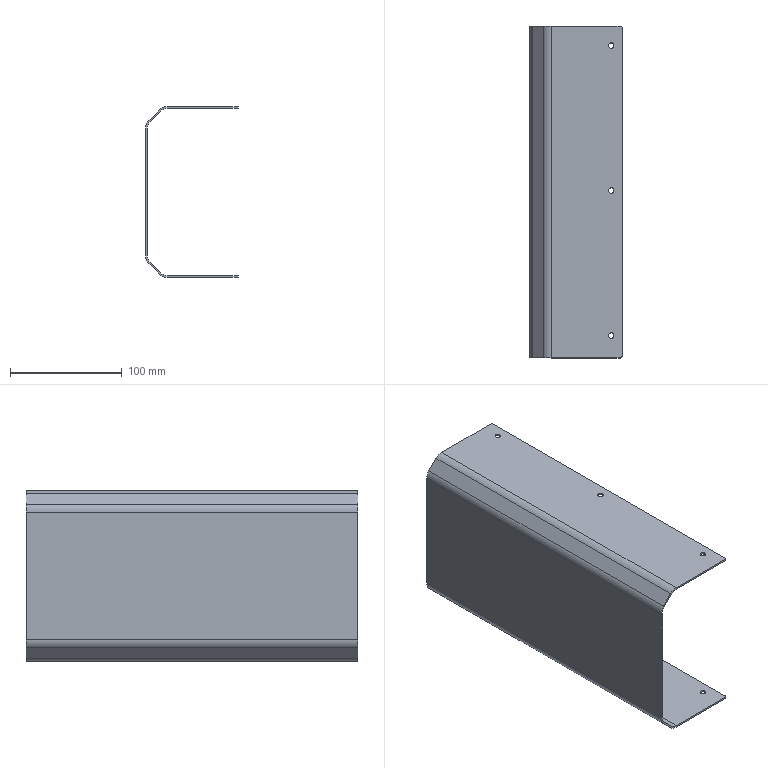Part | SolidWorks | features ICE 3, Fillet 2, Shell 2, Chamfer 1, Extrusion 1, HoleWzd 1 | 1 solid | 38 faces | box 83 x 297.5 x 153 mm | volume 132510 mm3 | cylinder 24 | plane 14 | commonest cylinder face diameters 5 x12 4 x4 17 x4 20 x4
STEP:
#1=CARTESIAN_POINT('',(29.,-17.5,75.));
#2=VERTEX_POINT('',#1);
#3=CARTESIAN_POINT('',(34.,-17.5,75.));
#4=VERTEX_POINT('',#3);
#5=CARTESIAN_POINT('',(31.5,-17.5,75.));
#6=DIRECTION('',(0.,0.,1.));
#7=DIRECTION('',(1.,0.,0.));
#8=AXIS2_PLACEMENT_3D('',#5,#6,#7);
#9=CIRCLE('',#8,2.5);
#10=EDGE_CURVE('',#2,#4,#9,.T.);
#11=ORIENTED_EDGE('',*,*,#10,.F.);
#12=CARTESIAN_POINT('',(29.,-17.5,76.5));
#13=VERTEX_POINT('',#12);
#14=CARTESIAN_POINT('',(29.,-17.5,76.5));
#15=DIRECTION('',(0.,0.,1.));
#16=VECTOR('',#15,1000.);
#17=LINE('',#14,#16);
#18=EDGE_CURVE('',#2,#13,#17,.T.);
#19=ORIENTED_EDGE('',*,*,#18,.T.);
#20=CARTESIAN_POINT('',(34.,-17.5,76.5));
#21=VERTEX_POINT('',#20);
#22=CARTESIAN_POINT('',(31.5,-17.5,76.5));
#23=DIRECTION('',(0.,0.,1.));
#24=DIRECTION('',(1.,0.,0.));
#25=AXIS2_PLACEMENT_3D('',#22,#23,#24);
#26=CIRCLE('',#25,2.5);
#27=EDGE_CURVE('',#13,#21,#26,.T.);
#28=ORIENTED_EDGE('',*,*,#27,.T.);
#29=CARTESIAN_POINT('',(34.,-17.5,76.5));
#30=DIRECTION('',(0.,0.,1.));
#31=VECTOR('',#30,1000.);
#32=LINE('',#29,#31);
#33=EDGE_CURVE('',#4,#21,#32,.T.);
#34=ORIENTED_EDGE('',*,*,#33,.F.);
#35=EDGE_LOOP('',(#11,#19,#28,#34));
#36=FACE_OUTER_BOUND('',#35,.T.);
#37=CARTESIAN_POINT('',(31.5,-17.5,76.5));
#38=DIRECTION('',(0.,0.,1.));
#39=DIRECTION('',(1.,0.,0.));
#40=AXIS2_PLACEMENT_3D('',#37,#38,#39);
#41=CYLINDRICAL_SURFACE('',#40,2.5);
#42=ADVANCED_FACE('',(#36),#41,.F.);
#43=CARTESIAN_POINT('',(29.,-17.5,-76.5));
#44=VERTEX_POINT('',#43);
#45=CARTESIAN_POINT('',(34.,-17.5,-76.5));
#46=VERTEX_POINT('',#45);
#47=CARTESIAN_POINT('',(31.5,-17.5,-76.5));
#48=DIRECTION('',(0.,0.,1.));
#49=DIRECTION('',(1.,0.,0.));
#50=AXIS2_PLACEMENT_3D('',#47,#48,#49);
#51=CIRCLE('',#50,2.5);
#52=EDGE_CURVE('',#44,#46,#51,.T.);
#53=ORIENTED_EDGE('',*,*,#52,.F.);
#54=CARTESIAN_POINT('',(29.,-17.5,-75.));
#55=VERTEX_POINT('',#54);
#56=CARTESIAN_POINT('',(29.,-17.5,76.5));
#57=DIRECTION('',(0.,0.,1.));
#58=VECTOR('',#57,1000.);
#59=LINE('',#56,#58);
#60=EDGE_CURVE('',#44,#55,#59,.T.);
#61=ORIENTED_EDGE('',*,*,#60,.T.);
#62=CARTESIAN_POINT('',(34.,-17.5,-75.));
#63=VERTEX_POINT('',#62);
#64=CARTESIAN_POINT('',(31.5,-17.5,-75.));
#65=DIRECTION('',(0.,0.,-1.));
#66=DIRECTION('',(-1.,0.,0.));
#67=AXIS2_PLACEMENT_3D('',#64,#65,#66);
#68=CIRCLE('',#67,2.5);
#69=EDGE_CURVE('',#63,#55,#68,.T.);
#70=ORIENTED_EDGE('',*,*,#69,.F.);
#71=CARTESIAN_POINT('',(34.,-17.5,76.5));
#72=DIRECTION('',(0.,0.,1.));
#73=VECTOR('',#72,1000.);
#74=LINE('',#71,#73);
#75=EDGE_CURVE('',#46,#63,#74,.T.);
#76=ORIENTED_EDGE('',*,*,#75,.F.);
#77=EDGE_LOOP('',(#53,#61,#70,#76));
#78=FACE_OUTER_BOUND('',#77,.T.);
#79=CARTESIAN_POINT('',(31.5,-17.5,76.5));
#80=DIRECTION('',(0.,0.,1.));
#81=DIRECTION('',(1.,0.,0.));
#82=AXIS2_PLACEMENT_3D('',#79,#80,#81);
#83=CYLINDRICAL_SURFACE('',#82,2.5);
#84=ADVANCED_FACE('',(#78),#83,.F.);
#85=CARTESIAN_POINT('',(29.,-147.5,75.));
#86=VERTEX_POINT('',#85);
#87=CARTESIAN_POINT('',(34.,-147.5,75.));
#88=VERTEX_POINT('',#87);
#89=CARTESIAN_POINT('',(31.5,-147.5,75.));
#90=DIRECTION('',(0.,0.,1.));
#91=DIRECTION('',(1.,0.,0.));
#92=AXIS2_PLACEMENT_3D('',#89,#90,#91);
#93=CIRCLE('',#92,2.5);
#94=EDGE_CURVE('',#86,#88,#93,.T.);
#95=ORIENTED_EDGE('',*,*,#94,.F.);
#96=CARTESIAN_POINT('',(29.,-147.5,76.5));
#97=VERTEX_POINT('',#96);
#98=CARTESIAN_POINT('',(29.,-147.5,76.5));
#99=DIRECTION('',(0.,0.,1.));
#100=VECTOR('',#99,1000.);
#101=LINE('',#98,#100);
#102=EDGE_CURVE('',#86,#97,#101,.T.);
#103=ORIENTED_EDGE('',*,*,#102,.T.);
#104=CARTESIAN_POINT('',(34.,-147.5,76.5));
#105=VERTEX_POINT('',#104);
#106=CARTESIAN_POINT('',(31.5,-147.5,76.5));
#107=DIRECTION('',(0.,0.,1.));
#108=DIRECTION('',(1.,0.,0.));
#109=AXIS2_PLACEMENT_3D('',#106,#107,#108);
#110=CIRCLE('',#109,2.5);
#111=EDGE_CURVE('',#97,#105,#110,.T.);
#112=ORIENTED_EDGE('',*,*,#111,.T.);
#113=CARTESIAN_POINT('',(34.,-147.5,76.5));
#114=DIRECTION('',(0.,0.,1.));
#115=VECTOR('',#114,1000.);
#116=LINE('',#113,#115);
#117=EDGE_CURVE('',#88,#105,#116,.T.);
#118=ORIENTED_EDGE('',*,*,#117,.F.);
#119=EDGE_LOOP('',(#95,#103,#112,#118));
#120=FACE_OUTER_BOUND('',#119,.T.);
#121=CARTESIAN_POINT('',(31.5,-147.5,76.5));
#122=DIRECTION('',(0.,0.,1.));
#123=DIRECTION('',(1.,0.,0.));
#124=AXIS2_PLACEMENT_3D('',#121,#122,#123);
#125=CYLINDRICAL_SURFACE('',#124,2.5);
#126=ADVANCED_FACE('',(#120),#125,.F.);
#127=CARTESIAN_POINT('',(29.,-147.5,-76.5));
#128=VERTEX_POINT('',#127);
#129=CARTESIAN_POINT('',(34.,-147.5,-76.5));
#130=VERTEX_POINT('',#129);
#131=CARTESIAN_POINT('',(31.5,-147.5,-76.5));
#132=DIRECTION('',(0.,0.,1.));
#133=DIRECTION('',(1.,0.,0.));
#134=AXIS2_PLACEMENT_3D('',#131,#132,#133);
#135=CIRCLE('',#134,2.5);
#136=EDGE_CURVE('',#128,#130,#135,.T.);
#137=ORIENTED_EDGE('',*,*,#136,.F.);
#138=CARTESIAN_POINT('',(29.,-147.5,-75.));
#139=VERTEX_POINT('',#138);
#140=CARTESIAN_POINT('',(29.,-147.5,76.5));
#141=DIRECTION('',(0.,0.,1.));
#142=VECTOR('',#141,1000.);
#143=LINE('',#140,#142);
#144=EDGE_CURVE('',#128,#139,#143,.T.);
#145=ORIENTED_EDGE('',*,*,#144,.T.);
#146=CARTESIAN_POINT('',(34.,-147.5,-75.));
#147=VERTEX_POINT('',#146);
#148=CARTESIAN_POINT('',(31.5,-147.5,-75.));
#149=DIRECTION('',(0.,0.,-1.));
#150=DIRECTION('',(-1.,0.,0.));
#151=AXIS2_PLACEMENT_3D('',#148,#149,#150);
#152=CIRCLE('',#151,2.5);
#153=EDGE_CURVE('',#147,#139,#152,.T.);
#154=ORIENTED_EDGE('',*,*,#153,.F.);
#155=CARTESIAN_POINT('',(34.,-147.5,76.5));
#156=DIRECTION('',(0.,0.,1.));
#157=VECTOR('',#156,1000.);
#158=LINE('',#155,#157);
#159=EDGE_CURVE('',#130,#147,#158,.T.);
#160=ORIENTED_EDGE('',*,*,#159,.F.);
#161=EDGE_LOOP('',(#137,#145,#154,#160));
#162=FACE_OUTER_BOUND('',#161,.T.);
#163=CARTESIAN_POINT('',(31.5,-147.5,76.5));
#164=DIRECTION('',(0.,0.,1.));
#165=DIRECTION('',(1.,0.,0.));
#166=AXIS2_PLACEMENT_3D('',#163,#164,#165);
#167=CYLINDRICAL_SURFACE('',#166,2.5);
#168=ADVANCED_FACE('',(#162),#167,.F.);
#169=CARTESIAN_POINT('',(29.,-277.5,75.));
#170=VERTEX_POINT('',#169);
#171=CARTESIAN_POINT('',(34.,-277.5,75.));
#172=VERTEX_POINT('',#171);
#173=CARTESIAN_POINT('',(31.5,-277.5,75.));
#174=DIRECTION('',(0.,0.,1.));
#175=DIRECTION('',(1.,0.,0.));
#176=AXIS2_PLACEMENT_3D('',#173,#174,#175);
#177=CIRCLE('',#176,2.5);
#178=EDGE_CURVE('',#170,#172,#177,.T.);
#179=ORIENTED_EDGE('',*,*,#178,.F.);
#180=CARTESIAN_POINT('',(29.,-277.5,76.5));
#181=VERTEX_POINT('',#180);
#182=CARTESIAN_POINT('',(29.,-277.5,76.5));
#183=DIRECTION('',(0.,0.,1.));
#184=VECTOR('',#183,1000.);
#185=LINE('',#182,#184);
#186=EDGE_CURVE('',#170,#181,#185,.T.);
#187=ORIENTED_EDGE('',*,*,#186,.T.);
#188=CARTESIAN_POINT('',(34.,-277.5,76.5));
#189=VERTEX_POINT('',#188);
#190=CARTESIAN_POINT('',(31.5,-277.5,76.5));
#191=DIRECTION('',(0.,0.,1.));
#192=DIRECTION('',(1.,0.,0.));
#193=AXIS2_PLACEMENT_3D('',#190,#191,#192);
#194=CIRCLE('',#193,2.5);
#195=EDGE_CURVE('',#181,#189,#194,.T.);
#196=ORIENTED_EDGE('',*,*,#195,.T.);
#197=CARTESIAN_POINT('',(34.,-277.5,76.5));
#198=DIRECTION('',(0.,0.,1.));
#199=VECTOR('',#198,1000.);
#200=LINE('',#197,#199);
#201=EDGE_CURVE('',#172,#189,#200,.T.);
#202=ORIENTED_EDGE('',*,*,#201,.F.);
#203=EDGE_LOOP('',(#179,#187,#196,#202));
#204=FACE_OUTER_BOUND('',#203,.T.);
#205=CARTESIAN_POINT('',(31.5,-277.5,76.5));
#206=DIRECTION('',(0.,0.,1.));
#207=DIRECTION('',(1.,0.,0.));
#208=AXIS2_PLACEMENT_3D('',#205,#206,#207);
#209=CYLINDRICAL_SURFACE('',#208,2.5);
#210=ADVANCED_FACE('',(#204),#209,.F.);
#211=CARTESIAN_POINT('',(29.,-277.5,-76.5));
#212=VERTEX_POINT('',#211);
#213=CARTESIAN_POINT('',(34.,-277.5,-76.5));
#214=VERTEX_POINT('',#213);
#215=CARTESIAN_POINT('',(31.5,-277.5,-76.5));
#216=DIRECTION('',(0.,0.,1.));
#217=DIRECTION('',(1.,0.,0.));
#218=AXIS2_PLACEMENT_3D('',#215,#216,#217);
#219=CIRCLE('',#218,2.5);
#220=EDGE_CURVE('',#212,#214,#219,.T.);
#221=ORIENTED_EDGE('',*,*,#220,.F.);
#222=CARTESIAN_POINT('',(29.,-277.5,-75.));
#223=VERTEX_POINT('',#222);
#224=CARTESIAN_POINT('',(29.,-277.5,76.5));
#225=DIRECTION('',(0.,0.,1.));
#226=VECTOR('',#225,1000.);
#227=LINE('',#224,#226);
#228=EDGE_CURVE('',#212,#223,#227,.T.);
#229=ORIENTED_EDGE('',*,*,#228,.T.);
#230=CARTESIAN_POINT('',(34.,-277.5,-75.));
#231=VERTEX_POINT('',#230);
#232=CARTESIAN_POINT('',(31.5,-277.5,-75.));
#233=DIRECTION('',(0.,0.,-1.));
#234=DIRECTION('',(-1.,0.,0.));
#235=AXIS2_PLACEMENT_3D('',#232,#233,#234);
#236=CIRCLE('',#235,2.5);
#237=EDGE_CURVE('',#231,#223,#236,.T.);
#238=ORIENTED_EDGE('',*,*,#237,.F.);
#239=CARTESIAN_POINT('',(34.,-277.5,76.5));
#240=DIRECTION('',(0.,0.,1.));
#241=VECTOR('',#240,1000.);
#242=LINE('',#239,#241);
#243=EDGE_CURVE('',#214,#231,#242,.T.);
#244=ORIENTED_EDGE('',*,*,#243,.F.);
#245=EDGE_LOOP('',(#221,#229,#238,#244));
#246=FACE_OUTER_BOUND('',#245,.T.);
#247=CARTESIAN_POINT('',(31.5,-277.5,76.5));
#248=DIRECTION('',(0.,0.,1.));
#249=DIRECTION('',(1.,0.,0.));
#250=AXIS2_PLACEMENT_3D('',#247,#248,#249);
#251=CYLINDRICAL_SURFACE('',#250,2.5);
#252=ADVANCED_FACE('',(#246),#251,.F.);
#253=CARTESIAN_POINT('',(41.5,-295.5,76.5));
#254=VERTEX_POINT('',#253);
#255=CARTESIAN_POINT('',(41.5,-2.,76.5));
#256=VERTEX_POINT('',#255);
#257=CARTESIAN_POINT('',(41.5,-297.5,76.5));
#258=DIRECTION('',(0.,1.,0.));
#259=VECTOR('',#258,1000.);
#260=LINE('',#257,#259);
#261=EDGE_CURVE('',#254,#256,#260,.T.);
#262=ORIENTED_EDGE('',*,*,#261,.F.);
#263=CARTESIAN_POINT('',(41.5,-295.5,75.));
#264=VERTEX_POINT('',#263);
#265=CARTESIAN_POINT('',(41.5,-295.5,75.));
#266=DIRECTION('',(0.,0.,-1.));
#267=VECTOR('',#266,1000.);
#268=LINE('',#265,#267);
#269=EDGE_CURVE('',#254,#264,#268,.T.);
#270=ORIENTED_EDGE('',*,*,#269,.T.);
#271=CARTESIAN_POINT('',(41.5,-2.,75.));
#272=VERTEX_POINT('',#271);
#273=CARTESIAN_POINT('',(41.5,-297.5,75.));
#274=DIRECTION('',(0.,1.,0.));
#275=VECTOR('',#274,1000.);
#276=LINE('',#273,#275);
#277=EDGE_CURVE('',#264,#272,#276,.T.);
#278=ORIENTED_EDGE('',*,*,#277,.T.);
#279=CARTESIAN_POINT('',(41.5,-2.,-76.5));
#280=DIRECTION('',(0.,0.,1.));
#281=VECTOR('',#280,1000.);
#282=LINE('',#279,#281);
#283=EDGE_CURVE('',#272,#256,#282,.T.);
#284=ORIENTED_EDGE('',*,*,#283,.T.);
#285=EDGE_LOOP('',(#262,#270,#278,#284));
#286=FACE_OUTER_BOUND('',#285,.T.);
#287=CARTESIAN_POINT('',(41.5,-297.5,-76.5));
#288=DIRECTION('',(1.,0.,0.));
#289=DIRECTION('',(0.,0.,-1.));
#290=AXIS2_PLACEMENT_3D('',#287,#288,#289);
#291=PLANE('',#290);
#292=ADVANCED_FACE('',(#286),#291,.T.);
#293=CARTESIAN_POINT('',(41.5,-295.5,-75.));
#294=VERTEX_POINT('',#293);
#295=CARTESIAN_POINT('',(41.5,-2.,-75.));
#296=VERTEX_POINT('',#295);
#297=CARTESIAN_POINT('',(41.5,-297.5,-75.));
#298=DIRECTION('',(0.,1.,0.));
#299=VECTOR('',#298,1000.);
#300=LINE('',#297,#299);
#301=EDGE_CURVE('',#294,#296,#300,.T.);
#302=ORIENTED_EDGE('',*,*,#301,.F.);
#303=CARTESIAN_POINT('',(41.5,-295.5,-76.5));
#304=VERTEX_POINT('',#303);
#305=CARTESIAN_POINT('',(41.5,-295.5,-76.5));
#306=DIRECTION('',(0.,0.,-1.));
#307=VECTOR('',#306,1000.);
#308=LINE('',#305,#307);
#309=EDGE_CURVE('',#294,#304,#308,.T.);
#310=ORIENTED_EDGE('',*,*,#309,.T.);
#311=CARTESIAN_POINT('',(41.5,-2.,-76.5));
#312=VERTEX_POINT('',#311);
#313=CARTESIAN_POINT('',(41.5,-297.5,-76.5));
#314=DIRECTION('',(0.,1.,0.));
#315=VECTOR('',#314,1000.);
#316=LINE('',#313,#315);
#317=EDGE_CURVE('',#304,#312,#316,.T.);
#318=ORIENTED_EDGE('',*,*,#317,.T.);
#319=CARTESIAN_POINT('',(41.5,-2.,-76.5));
#320=DIRECTION('',(0.,0.,1.));
#321=VECTOR('',#320,1000.);
#322=LINE('',#319,#321);
#323=EDGE_CURVE('',#312,#296,#322,.T.);
#324=ORIENTED_EDGE('',*,*,#323,.T.);
#325=EDGE_LOOP('',(#302,#310,#318,#324));
#326=FACE_OUTER_BOUND('',#325,.T.);
#327=CARTESIAN_POINT('',(41.5,-297.5,-76.5));
#328=DIRECTION('',(1.,0.,0.));
#329=DIRECTION('',(0.,0.,-1.));
#330=AXIS2_PLACEMENT_3D('',#327,#328,#329);
#331=PLANE('',#330);
#332=ADVANCED_FACE('',(#326),#331,.T.);
#333=CARTESIAN_POINT('',(31.5,-17.5,76.5));
#334=DIRECTION('',(0.,0.,1.));
#335=DIRECTION('',(1.,0.,0.));
#336=AXIS2_PLACEMENT_3D('',#333,#334,#335);
#337=CIRCLE('',#336,2.5);
#338=EDGE_CURVE('',#21,#13,#337,.T.);
#339=ORIENTED_EDGE('',*,*,#338,.F.);
#340=ORIENTED_EDGE('',*,*,#27,.F.);
#341=EDGE_LOOP('',(#339,#340));
#342=FACE_BOUND('',#341,.T.);
#343=CARTESIAN_POINT('',(31.5,-147.5,76.5));
#344=DIRECTION('',(0.,0.,1.));
#345=DIRECTION('',(1.,0.,0.));
#346=AXIS2_PLACEMENT_3D('',#343,#344,#345);
#347=CIRCLE('',#346,2.5);
#348=EDGE_CURVE('',#105,#97,#347,.T.);
#349=ORIENTED_EDGE('',*,*,#348,.F.);
#350=ORIENTED_EDGE('',*,*,#111,.F.);
#351=EDGE_LOOP('',(#349,#350));
#352=FACE_BOUND('',#351,.T.);
#353=CARTESIAN_POINT('',(31.5,-277.5,76.5));
#354=DIRECTION('',(0.,0.,1.));
#355=DIRECTION('',(1.,0.,0.));
#356=AXIS2_PLACEMENT_3D('',#353,#354,#355);
#357=CIRCLE('',#356,2.5);
#358=EDGE_CURVE('',#189,#181,#357,.T.);
#359=ORIENTED_EDGE('',*,*,#358,.F.);
#360=ORIENTED_EDGE('',*,*,#195,.F.);
#361=EDGE_LOOP('',(#359,#360));
#362=FACE_BOUND('',#361,.T.);
#363=CARTESIAN_POINT('',(-22.358,-297.5,76.5));
#364=VERTEX_POINT('',#363);
#365=CARTESIAN_POINT('',(39.5,-297.5,76.5));
#366=VERTEX_POINT('',#365);
#367=CARTESIAN_POINT('',(-41.5,-297.5,76.5));
#368=DIRECTION('',(1.,0.,0.));
#369=VECTOR('',#368,1000.);
#370=LINE('',#367,#369);
#371=EDGE_CURVE('',#364,#366,#370,.T.);
#372=ORIENTED_EDGE('',*,*,#371,.T.);
#373=CARTESIAN_POINT('',(39.5,-295.5,76.5));
#374=DIRECTION('',(0.,0.,1.));
#375=DIRECTION('',(1.,0.,0.));
#376=AXIS2_PLACEMENT_3D('',#373,#374,#375);
#377=CIRCLE('',#376,2.);
#378=EDGE_CURVE('',#366,#254,#377,.T.);
#379=ORIENTED_EDGE('',*,*,#378,.T.);
#380=ORIENTED_EDGE('',*,*,#261,.T.);
#381=CARTESIAN_POINT('',(39.5,0.,76.5));
#382=VERTEX_POINT('',#381);
#383=CARTESIAN_POINT('',(39.5,-2.,76.5));
#384=DIRECTION('',(0.,0.,1.));
#385=DIRECTION('',(1.,0.,0.));
#386=AXIS2_PLACEMENT_3D('',#383,#384,#385);
#387=CIRCLE('',#386,2.);
#388=EDGE_CURVE('',#256,#382,#387,.T.);
#389=ORIENTED_EDGE('',*,*,#388,.T.);
#390=CARTESIAN_POINT('',(-22.358,0.,76.5));
#391=VERTEX_POINT('',#390);
#392=CARTESIAN_POINT('',(-41.5,0.,76.5));
#393=DIRECTION('',(1.,0.,0.));
#394=VECTOR('',#393,1000.);
#395=LINE('',#392,#394);
#396=EDGE_CURVE('',#391,#382,#395,.T.);
#397=ORIENTED_EDGE('',*,*,#396,.F.);
#398=CARTESIAN_POINT('',(-22.358,-297.5,76.5));
#399=DIRECTION('',(0.,-1.,0.));
#400=VECTOR('',#399,1000.);
#401=LINE('',#398,#400);
#402=EDGE_CURVE('',#391,#364,#401,.T.);
#403=ORIENTED_EDGE('',*,*,#402,.T.);
#404=EDGE_LOOP('',(#372,#379,#380,#389,#397,#403));
#405=FACE_OUTER_BOUND('',#404,.T.);
#406=CARTESIAN_POINT('',(-41.5,-297.5,76.5));
#407=DIRECTION('',(0.,0.,1.));
#408=DIRECTION('',(1.,0.,0.));
#409=AXIS2_PLACEMENT_3D('',#406,#407,#408);
#410=PLANE('',#409);
#411=ADVANCED_FACE('',(#342,#352,#362,#405),#410,.T.);
#412=CARTESIAN_POINT('',(-41.5,0.,-57.358));
#413=VERTEX_POINT('',#412);
#414=CARTESIAN_POINT('',(-41.5,0.,57.358));
#415=VERTEX_POINT('',#414);
#416=CARTESIAN_POINT('',(-41.5,0.,-76.5));
#417=DIRECTION('',(0.,0.,1.));
#418=VECTOR('',#417,1000.);
#419=LINE('',#416,#418);
#420=EDGE_CURVE('',#413,#415,#419,.T.);
#421=ORIENTED_EDGE('',*,*,#420,.F.);
#422=CARTESIAN_POINT('',(-41.5,-297.5,-57.358));
#423=VERTEX_POINT('',#422);
#424=CARTESIAN_POINT('',(-41.5,-297.5,-57.358));
#425=DIRECTION('',(0.,-1.,0.));
#426=VECTOR('',#425,1000.);
#427=LINE('',#424,#426);
#428=EDGE_CURVE('',#413,#423,#427,.T.);
#429=ORIENTED_EDGE('',*,*,#428,.T.);
#430=CARTESIAN_POINT('',(-41.5,-297.5,57.358));
#431=VERTEX_POINT('',#430);
#432=CARTESIAN_POINT('',(-41.5,-297.5,-76.5));
#433=DIRECTION('',(0.,0.,1.));
#434=VECTOR('',#433,1000.);
#435=LINE('',#432,#434);
#436=EDGE_CURVE('',#423,#431,#435,.T.);
#437=ORIENTED_EDGE('',*,*,#436,.T.);
#438=CARTESIAN_POINT('',(-41.5,-297.5,57.358));
#439=DIRECTION('',(0.,1.,0.));
#440=VECTOR('',#439,1000.);
#441=LINE('',#438,#440);
#442=EDGE_CURVE('',#431,#415,#441,.T.);
#443=ORIENTED_EDGE('',*,*,#442,.T.);
#444=EDGE_LOOP('',(#421,#429,#437,#443));
#445=FACE_OUTER_BOUND('',#444,.T.);
#446=CARTESIAN_POINT('',(-41.5,-297.5,-76.5));
#447=DIRECTION('',(-1.,0.,0.));
#448=DIRECTION('',(0.,0.,1.));
#449=AXIS2_PLACEMENT_3D('',#446,#447,#448);
#450=PLANE('',#449);
#451=ADVANCED_FACE('',(#445),#450,.T.);
#452=CARTESIAN_POINT('',(31.5,-17.5,-76.5));
#453=DIRECTION('',(0.,0.,1.));
#454=DIRECTION('',(1.,0.,0.));
#455=AXIS2_PLACEMENT_3D('',#452,#453,#454);
#456=CIRCLE('',#455,2.5);
#457=EDGE_CURVE('',#46,#44,#456,.T.);
#458=ORIENTED_EDGE('',*,*,#457,.T.);
#459=ORIENTED_EDGE('',*,*,#52,.T.);
#460=EDGE_LOOP('',(#458,#459));
#461=FACE_BOUND('',#460,.T.);
#462=CARTESIAN_POINT('',(31.5,-147.5,-76.5));
#463=DIRECTION('',(0.,0.,1.));
#464=DIRECTION('',(1.,0.,0.));
#465=AXIS2_PLACEMENT_3D('',#462,#463,#464);
#466=CIRCLE('',#465,2.5);
#467=EDGE_CURVE('',#130,#128,#466,.T.);
#468=ORIENTED_EDGE('',*,*,#467,.T.);
#469=ORIENTED_EDGE('',*,*,#136,.T.);
#470=EDGE_LOOP('',(#468,#469));
#471=FACE_BOUND('',#470,.T.);
#472=CARTESIAN_POINT('',(31.5,-277.5,-76.5));
#473=DIRECTION('',(0.,0.,1.));
#474=DIRECTION('',(1.,0.,0.));
#475=AXIS2_PLACEMENT_3D('',#472,#473,#474);
#476=CIRCLE('',#475,2.5);
#477=EDGE_CURVE('',#214,#212,#476,.T.);
#478=ORIENTED_EDGE('',*,*,#477,.T.);
#479=ORIENTED_EDGE('',*,*,#220,.T.);
#480=EDGE_LOOP('',(#478,#479));
#481=FACE_BOUND('',#480,.T.);
#482=ORIENTED_EDGE('',*,*,#317,.F.);
#483=CARTESIAN_POINT('',(39.5,-297.5,-76.5));
#484=VERTEX_POINT('',#483);
#485=CARTESIAN_POINT('',(39.5,-295.5,-76.5));
#486=DIRECTION('',(0.,0.,-1.));
#487=DIRECTION('',(-1.,0.,0.));
#488=AXIS2_PLACEMENT_3D('',#485,#486,#487);
#489=CIRCLE('',#488,2.);
#490=EDGE_CURVE('',#304,#484,#489,.T.);
#491=ORIENTED_EDGE('',*,*,#490,.T.);
#492=CARTESIAN_POINT('',(-22.358,-297.5,-76.5));
#493=VERTEX_POINT('',#492);
#494=CARTESIAN_POINT('',(-41.5,-297.5,-76.5));
#495=DIRECTION('',(-1.,0.,0.));
#496=VECTOR('',#495,1000.);
#497=LINE('',#494,#496);
#498=EDGE_CURVE('',#484,#493,#497,.T.);
#499=ORIENTED_EDGE('',*,*,#498,.T.);
#500=CARTESIAN_POINT('',(-22.358,0.,-76.5));
#501=VERTEX_POINT('',#500);
#502=CARTESIAN_POINT('',(-22.358,-297.5,-76.5));
#503=DIRECTION('',(0.,1.,0.));
#504=VECTOR('',#503,1000.);
#505=LINE('',#502,#504);
#506=EDGE_CURVE('',#493,#501,#505,.T.);
#507=ORIENTED_EDGE('',*,*,#506,.T.);
#508=CARTESIAN_POINT('',(39.5,0.,-76.5));
#509=VERTEX_POINT('',#508);
#510=CARTESIAN_POINT('',(-41.5,0.,-76.5));
#511=DIRECTION('',(-1.,0.,0.));
#512=VECTOR('',#511,1000.);
#513=LINE('',#510,#512);
#514=EDGE_CURVE('',#509,#501,#513,.T.);
#515=ORIENTED_EDGE('',*,*,#514,.F.);
#516=CARTESIAN_POINT('',(39.5,-2.,-76.5));
#517=DIRECTION('',(0.,0.,-1.));
#518=DIRECTION('',(-1.,0.,0.));
#519=AXIS2_PLACEMENT_3D('',#516,#517,#518);
#520=CIRCLE('',#519,2.);
#521=EDGE_CURVE('',#509,#312,#520,.T.);
#522=ORIENTED_EDGE('',*,*,#521,.T.);
#523=EDGE_LOOP('',(#482,#491,#499,#507,#515,#522));
#524=FACE_OUTER_BOUND('',#523,.T.);
#525=CARTESIAN_POINT('',(-41.5,-297.5,-76.5));
#526=DIRECTION('',(0.,0.,-1.));
#527=DIRECTION('',(-1.,0.,0.));
#528=AXIS2_PLACEMENT_3D('',#525,#526,#527);
#529=PLANE('',#528);
#530=ADVANCED_FACE('',(#461,#471,#481,#524),#529,.T.);
#531=ORIENTED_EDGE('',*,*,#498,.F.);
#532=CARTESIAN_POINT('',(39.5,-297.5,-75.));
#533=VERTEX_POINT('',#532);
#534=CARTESIAN_POINT('',(39.5,-297.5,-75.));
#535=DIRECTION('',(0.,0.,1.));
#536=VECTOR('',#535,1000.);
#537=LINE('',#534,#536);
#538=EDGE_CURVE('',#484,#533,#537,.T.);
#539=ORIENTED_EDGE('',*,*,#538,.T.);
#540=CARTESIAN_POINT('',(-22.358,-297.5,-75.));
#541=VERTEX_POINT('',#540);
#542=CARTESIAN_POINT('',(0.,-297.5,-75.));
#543=DIRECTION('',(-1.,0.,0.));
#544=VECTOR('',#543,1000.);
#545=LINE('',#542,#544);
#546=EDGE_CURVE('',#533,#541,#545,.T.);
#547=ORIENTED_EDGE('',*,*,#546,.T.);
#548=CARTESIAN_POINT('',(-28.368,-297.5,-72.51));
#549=VERTEX_POINT('',#548);
#550=CARTESIAN_POINT('',(-22.358,-297.5,-66.5));
#551=DIRECTION('',(0.,-1.,0.));
#552=DIRECTION('',(0.,0.,1.));
#553=AXIS2_PLACEMENT_3D('',#550,#551,#552);
#554=CIRCLE('',#553,8.5);
#555=EDGE_CURVE('',#549,#541,#554,.T.);
#556=ORIENTED_EDGE('',*,*,#555,.F.);
#557=CARTESIAN_POINT('',(-37.51,-297.5,-63.368));
#558=VERTEX_POINT('',#557);
#559=CARTESIAN_POINT('',(-25.439,-297.5,-75.439));
#560=DIRECTION('',(0.7071,0.,-0.7071));
#561=VECTOR('',#560,1000.);
#562=LINE('',#559,#561);
#563=EDGE_CURVE('',#558,#549,#562,.T.);
#564=ORIENTED_EDGE('',*,*,#563,.F.);
#565=CARTESIAN_POINT('',(-40.,-297.5,-57.358));
#566=VERTEX_POINT('',#565);
#567=CARTESIAN_POINT('',(-31.5,-297.5,-57.358));
#568=DIRECTION('',(0.,-1.,0.));
#569=DIRECTION('',(0.,0.,1.));
#570=AXIS2_PLACEMENT_3D('',#567,#568,#569);
#571=CIRCLE('',#570,8.5);
#572=EDGE_CURVE('',#566,#558,#571,.T.);
#573=ORIENTED_EDGE('',*,*,#572,.F.);
#574=CARTESIAN_POINT('',(-40.,-297.5,57.358));
#575=VERTEX_POINT('',#574);
#576=CARTESIAN_POINT('',(-40.,-297.5,0.));
#577=DIRECTION('',(0.,0.,1.));
#578=VECTOR('',#577,1000.);
#579=LINE('',#576,#578);
#580=EDGE_CURVE('',#566,#575,#579,.T.);
#581=ORIENTED_EDGE('',*,*,#580,.T.);
#582=CARTESIAN_POINT('',(-37.51,-297.5,63.368));
#583=VERTEX_POINT('',#582);
#584=CARTESIAN_POINT('',(-31.5,-297.5,57.358));
#585=DIRECTION('',(0.,-1.,0.));
#586=DIRECTION('',(0.,0.,1.));
#587=AXIS2_PLACEMENT_3D('',#584,#585,#586);
#588=CIRCLE('',#587,8.5);
#589=EDGE_CURVE('',#583,#575,#588,.T.);
#590=ORIENTED_EDGE('',*,*,#589,.F.);
#591=CARTESIAN_POINT('',(-28.368,-297.5,72.51));
#592=VERTEX_POINT('',#591);
#593=CARTESIAN_POINT('',(-40.439,-297.5,60.439));
#594=DIRECTION('',(-0.7071,0.,-0.7071));
#595=VECTOR('',#594,1000.);
#596=LINE('',#593,#595);
#597=EDGE_CURVE('',#592,#583,#596,.T.);
#598=ORIENTED_EDGE('',*,*,#597,.F.);
#599=CARTESIAN_POINT('',(-22.358,-297.5,75.));
#600=VERTEX_POINT('',#599);
#601=CARTESIAN_POINT('',(-22.358,-297.5,66.5));
#602=DIRECTION('',(0.,-1.,0.));
#603=DIRECTION('',(0.,0.,1.));
#604=AXIS2_PLACEMENT_3D('',#601,#602,#603);
#605=CIRCLE('',#604,8.5);
#606=EDGE_CURVE('',#600,#592,#605,.T.);
#607=ORIENTED_EDGE('',*,*,#606,.F.);
#608=CARTESIAN_POINT('',(39.5,-297.5,75.));
#609=VERTEX_POINT('',#608);
#610=CARTESIAN_POINT('',(0.,-297.5,75.));
#611=DIRECTION('',(1.,0.,0.));
#612=VECTOR('',#611,1000.);
#613=LINE('',#610,#612);
#614=EDGE_CURVE('',#600,#609,#613,.T.);
#615=ORIENTED_EDGE('',*,*,#614,.T.);
#616=CARTESIAN_POINT('',(39.5,-297.5,76.5));
#617=DIRECTION('',(0.,0.,1.));
#618=VECTOR('',#617,1000.);
#619=LINE('',#616,#618);
#620=EDGE_CURVE('',#609,#366,#619,.T.);
#621=ORIENTED_EDGE('',*,*,#620,.T.);
#622=ORIENTED_EDGE('',*,*,#371,.F.);
#623=CARTESIAN_POINT('',(-29.429,-297.5,73.571));
#624=VERTEX_POINT('',#623);
#625=CARTESIAN_POINT('',(-22.358,-297.5,66.5));
#626=DIRECTION('',(0.,-1.,0.));
#627=DIRECTION('',(0.,0.,1.));
#628=AXIS2_PLACEMENT_3D('',#625,#626,#627);
#629=CIRCLE('',#628,10.);
#630=EDGE_CURVE('',#364,#624,#629,.T.);
#631=ORIENTED_EDGE('',*,*,#630,.T.);
#632=CARTESIAN_POINT('',(-38.571,-297.5,64.429));
#633=VERTEX_POINT('',#632);
#634=CARTESIAN_POINT('',(-41.5,-297.5,61.5));
#635=DIRECTION('',(-0.7071,0.,-0.7071));
#636=VECTOR('',#635,1000.);
#637=LINE('',#634,#636);
#638=EDGE_CURVE('',#624,#633,#637,.T.);
#639=ORIENTED_EDGE('',*,*,#638,.T.);
#640=CARTESIAN_POINT('',(-31.5,-297.5,57.358));
#641=DIRECTION('',(0.,-1.,0.));
#642=DIRECTION('',(0.,0.,1.));
#643=AXIS2_PLACEMENT_3D('',#640,#641,#642);
#644=CIRCLE('',#643,10.);
#645=EDGE_CURVE('',#633,#431,#644,.T.);
#646=ORIENTED_EDGE('',*,*,#645,.T.);
#647=ORIENTED_EDGE('',*,*,#436,.F.);
#648=CARTESIAN_POINT('',(-38.571,-297.5,-64.429));
#649=VERTEX_POINT('',#648);
#650=CARTESIAN_POINT('',(-31.5,-297.5,-57.358));
#651=DIRECTION('',(0.,-1.,0.));
#652=DIRECTION('',(0.,0.,1.));
#653=AXIS2_PLACEMENT_3D('',#650,#651,#652);
#654=CIRCLE('',#653,10.);
#655=EDGE_CURVE('',#423,#649,#654,.T.);
#656=ORIENTED_EDGE('',*,*,#655,.T.);
#657=CARTESIAN_POINT('',(-29.429,-297.5,-73.571));
#658=VERTEX_POINT('',#657);
#659=CARTESIAN_POINT('',(-26.5,-297.5,-76.5));
#660=DIRECTION('',(0.7071,0.,-0.7071));
#661=VECTOR('',#660,1000.);
#662=LINE('',#659,#661);
#663=EDGE_CURVE('',#649,#658,#662,.T.);
#664=ORIENTED_EDGE('',*,*,#663,.T.);
#665=CARTESIAN_POINT('',(-22.358,-297.5,-66.5));
#666=DIRECTION('',(0.,-1.,0.));
#667=DIRECTION('',(0.,0.,1.));
#668=AXIS2_PLACEMENT_3D('',#665,#666,#667);
#669=CIRCLE('',#668,10.);
#670=EDGE_CURVE('',#658,#493,#669,.T.);
#671=ORIENTED_EDGE('',*,*,#670,.T.);
#672=EDGE_LOOP('',(#531,#539,#547,#556,#564,#573,#581,#590,#598,#607,#615,#621,#622,#631,#639,#646,#647,#656,#664,#671));
#673=FACE_OUTER_BOUND('',#672,.T.);
#674=CARTESIAN_POINT('',(0.,-297.5,0.));
#675=DIRECTION('',(0.,1.,0.));
#676=DIRECTION('',(0.,0.,1.));
#677=AXIS2_PLACEMENT_3D('',#674,#675,#676);
#678=PLANE('',#677);
#679=ADVANCED_FACE('',(#673),#678,.F.);
#680=ORIENTED_EDGE('',*,*,#396,.T.);
#681=CARTESIAN_POINT('',(39.5,0.,75.));
#682=VERTEX_POINT('',#681);
#683=CARTESIAN_POINT('',(39.5,0.,0.));
#684=DIRECTION('',(0.,0.,-1.));
#685=VECTOR('',#684,1000.);
#686=LINE('',#683,#685);
#687=EDGE_CURVE('',#382,#682,#686,.T.);
#688=ORIENTED_EDGE('',*,*,#687,.T.);
#689=CARTESIAN_POINT('',(-22.358,0.,75.));
#690=VERTEX_POINT('',#689);
#691=CARTESIAN_POINT('',(0.,0.,75.));
#692=DIRECTION('',(1.,0.,0.));
#693=VECTOR('',#692,1000.);
#694=LINE('',#691,#693);
#695=EDGE_CURVE('',#690,#682,#694,.T.);
#696=ORIENTED_EDGE('',*,*,#695,.F.);
#697=CARTESIAN_POINT('',(-28.368,0.,72.51));
#698=VERTEX_POINT('',#697);
#699=CARTESIAN_POINT('',(-22.358,0.,66.5));
#700=DIRECTION('',(0.,1.,0.));
#701=DIRECTION('',(0.,0.,1.));
#702=AXIS2_PLACEMENT_3D('',#699,#700,#701);
#703=CIRCLE('',#702,8.5);
#704=EDGE_CURVE('',#698,#690,#703,.T.);
#705=ORIENTED_EDGE('',*,*,#704,.F.);
#706=CARTESIAN_POINT('',(-37.51,0.,63.368));
#707=VERTEX_POINT('',#706);
#708=CARTESIAN_POINT('',(-50.439,0.,50.439));
#709=DIRECTION('',(0.7071,0.,0.7071));
#710=VECTOR('',#709,1000.);
#711=LINE('',#708,#710);
#712=EDGE_CURVE('',#707,#698,#711,.T.);
#713=ORIENTED_EDGE('',*,*,#712,.F.);
#714=CARTESIAN_POINT('',(-40.,0.,57.358));
#715=VERTEX_POINT('',#714);
#716=CARTESIAN_POINT('',(-31.5,0.,57.358));
#717=DIRECTION('',(0.,1.,0.));
#718=DIRECTION('',(0.,0.,1.));
#719=AXIS2_PLACEMENT_3D('',#716,#717,#718);
#720=CIRCLE('',#719,8.5);
#721=EDGE_CURVE('',#715,#707,#720,.T.);
#722=ORIENTED_EDGE('',*,*,#721,.F.);
#723=CARTESIAN_POINT('',(-40.,0.,-57.358));
#724=VERTEX_POINT('',#723);
#725=CARTESIAN_POINT('',(-40.,0.,0.));
#726=DIRECTION('',(0.,0.,1.));
#727=VECTOR('',#726,1000.);
#728=LINE('',#725,#727);
#729=EDGE_CURVE('',#724,#715,#728,.T.);
#730=ORIENTED_EDGE('',*,*,#729,.F.);
#731=CARTESIAN_POINT('',(-37.51,0.,-63.368));
#732=VERTEX_POINT('',#731);
#733=CARTESIAN_POINT('',(-31.5,0.,-57.358));
#734=DIRECTION('',(0.,1.,0.));
#735=DIRECTION('',(0.,0.,1.));
#736=AXIS2_PLACEMENT_3D('',#733,#734,#735);
#737=CIRCLE('',#736,8.5);
#738=EDGE_CURVE('',#732,#724,#737,.T.);
#739=ORIENTED_EDGE('',*,*,#738,.F.);
#740=CARTESIAN_POINT('',(-28.368,0.,-72.51));
#741=VERTEX_POINT('',#740);
#742=CARTESIAN_POINT('',(-50.439,0.,-50.439));
#743=DIRECTION('',(-0.7071,0.,0.7071));
#744=VECTOR('',#743,1000.);
#745=LINE('',#742,#744);
#746=EDGE_CURVE('',#741,#732,#745,.T.);
#747=ORIENTED_EDGE('',*,*,#746,.F.);
#748=CARTESIAN_POINT('',(-22.358,0.,-75.));
#749=VERTEX_POINT('',#748);
#750=CARTESIAN_POINT('',(-22.358,0.,-66.5));
#751=DIRECTION('',(0.,1.,0.));
#752=DIRECTION('',(0.,0.,1.));
#753=AXIS2_PLACEMENT_3D('',#750,#751,#752);
#754=CIRCLE('',#753,8.5);
#755=EDGE_CURVE('',#749,#741,#754,.T.);
#756=ORIENTED_EDGE('',*,*,#755,.F.);
#757=CARTESIAN_POINT('',(39.5,0.,-75.));
#758=VERTEX_POINT('',#757);
#759=CARTESIAN_POINT('',(0.,0.,-75.));
#760=DIRECTION('',(-1.,0.,0.));
#761=VECTOR('',#760,1000.);
#762=LINE('',#759,#761);
#763=EDGE_CURVE('',#758,#749,#762,.T.);
#764=ORIENTED_EDGE('',*,*,#763,.F.);
#765=CARTESIAN_POINT('',(39.5,0.,0.));
#766=DIRECTION('',(0.,0.,-1.));
#767=VECTOR('',#766,1000.);
#768=LINE('',#765,#767);
#769=EDGE_CURVE('',#758,#509,#768,.T.);
#770=ORIENTED_EDGE('',*,*,#769,.T.);
#771=ORIENTED_EDGE('',*,*,#514,.T.);
#772=CARTESIAN_POINT('',(-29.429,0.,-73.571));
#773=VERTEX_POINT('',#772);
#774=CARTESIAN_POINT('',(-22.358,0.,-66.5));
#775=DIRECTION('',(0.,1.,0.));
#776=DIRECTION('',(0.,0.,1.));
#777=AXIS2_PLACEMENT_3D('',#774,#775,#776);
#778=CIRCLE('',#777,10.);
#779=EDGE_CURVE('',#501,#773,#778,.T.);
#780=ORIENTED_EDGE('',*,*,#779,.T.);
#781=CARTESIAN_POINT('',(-38.571,0.,-64.429));
#782=VERTEX_POINT('',#781);
#783=CARTESIAN_POINT('',(-51.5,0.,-51.5));
#784=DIRECTION('',(-0.7071,0.,0.7071));
#785=VECTOR('',#784,1000.);
#786=LINE('',#783,#785);
#787=EDGE_CURVE('',#773,#782,#786,.T.);
#788=ORIENTED_EDGE('',*,*,#787,.T.);
#789=CARTESIAN_POINT('',(-31.5,0.,-57.358));
#790=DIRECTION('',(0.,1.,0.));
#791=DIRECTION('',(0.,0.,1.));
#792=AXIS2_PLACEMENT_3D('',#789,#790,#791);
#793=CIRCLE('',#792,10.);
#794=EDGE_CURVE('',#782,#413,#793,.T.);
#795=ORIENTED_EDGE('',*,*,#794,.T.);
#796=ORIENTED_EDGE('',*,*,#420,.T.);
#797=CARTESIAN_POINT('',(-38.571,0.,64.429));
#798=VERTEX_POINT('',#797);
#799=CARTESIAN_POINT('',(-31.5,0.,57.358));
#800=DIRECTION('',(0.,1.,0.));
#801=DIRECTION('',(0.,0.,1.));
#802=AXIS2_PLACEMENT_3D('',#799,#800,#801);
#803=CIRCLE('',#802,10.);
#804=EDGE_CURVE('',#415,#798,#803,.T.);
#805=ORIENTED_EDGE('',*,*,#804,.T.);
#806=CARTESIAN_POINT('',(-29.429,0.,73.571));
#807=VERTEX_POINT('',#806);
#808=CARTESIAN_POINT('',(-51.5,0.,51.5));
#809=DIRECTION('',(0.7071,0.,0.7071));
#810=VECTOR('',#809,1000.);
#811=LINE('',#808,#810);
#812=EDGE_CURVE('',#798,#807,#811,.T.);
#813=ORIENTED_EDGE('',*,*,#812,.T.);
#814=CARTESIAN_POINT('',(-22.358,0.,66.5));
#815=DIRECTION('',(0.,1.,0.));
#816=DIRECTION('',(0.,0.,1.));
#817=AXIS2_PLACEMENT_3D('',#814,#815,#816);
#818=CIRCLE('',#817,10.);
#819=EDGE_CURVE('',#807,#391,#818,.T.);
#820=ORIENTED_EDGE('',*,*,#819,.T.);
#821=EDGE_LOOP('',(#680,#688,#696,#705,#713,#722,#730,#739,#747,#756,#764,#770,#771,#780,#788,#795,#796,#805,#813,#820));
#822=FACE_OUTER_BOUND('',#821,.T.);
#823=CARTESIAN_POINT('',(0.,0.,0.));
#824=DIRECTION('',(0.,1.,0.));
#825=DIRECTION('',(0.,0.,1.));
#826=AXIS2_PLACEMENT_3D('',#823,#824,#825);
#827=PLANE('',#826);
#828=ADVANCED_FACE('',(#822),#827,.T.);
#829=ORIENTED_EDGE('',*,*,#663,.F.);
#830=CARTESIAN_POINT('',(-38.571,-297.5,-64.429));
#831=DIRECTION('',(0.,1.,0.));
#832=VECTOR('',#831,1000.);
#833=LINE('',#830,#832);
#834=EDGE_CURVE('',#649,#782,#833,.T.);
#835=ORIENTED_EDGE('',*,*,#834,.T.);
#836=ORIENTED_EDGE('',*,*,#787,.F.);
#837=CARTESIAN_POINT('',(-29.429,-297.5,-73.571));
#838=DIRECTION('',(0.,-1.,0.));
#839=VECTOR('',#838,1000.);
#840=LINE('',#837,#839);
#841=EDGE_CURVE('',#773,#658,#840,.T.);
#842=ORIENTED_EDGE('',*,*,#841,.T.);
#843=EDGE_LOOP('',(#829,#835,#836,#842));
#844=FACE_OUTER_BOUND('',#843,.T.);
#845=CARTESIAN_POINT('',(-26.5,-297.5,-76.5));
#846=DIRECTION('',(0.7071,0.,0.7071));
#847=DIRECTION('',(0.,1.,0.));
#848=AXIS2_PLACEMENT_3D('',#845,#846,#847);
#849=PLANE('',#848);
#850=ADVANCED_FACE('',(#844),#849,.F.);
#851=ORIENTED_EDGE('',*,*,#812,.F.);
#852=CARTESIAN_POINT('',(-38.571,-297.5,64.429));
#853=DIRECTION('',(0.,-1.,0.));
#854=VECTOR('',#853,1000.);
#855=LINE('',#852,#854);
#856=EDGE_CURVE('',#798,#633,#855,.T.);
#857=ORIENTED_EDGE('',*,*,#856,.T.);
#858=ORIENTED_EDGE('',*,*,#638,.F.);
#859=CARTESIAN_POINT('',(-29.429,-297.5,73.571));
#860=DIRECTION('',(0.,1.,0.));
#861=VECTOR('',#860,1000.);
#862=LINE('',#859,#861);
#863=EDGE_CURVE('',#624,#807,#862,.T.);
#864=ORIENTED_EDGE('',*,*,#863,.T.);
#865=EDGE_LOOP('',(#851,#857,#858,#864));
#866=FACE_OUTER_BOUND('',#865,.T.);
#867=CARTESIAN_POINT('',(-41.5,-297.5,61.5));
#868=DIRECTION('',(0.7071,0.,-0.7071));
#869=DIRECTION('',(0.,1.,0.));
#870=AXIS2_PLACEMENT_3D('',#867,#868,#869);
#871=PLANE('',#870);
#872=ADVANCED_FACE('',(#866),#871,.F.);
#873=ORIENTED_EDGE('',*,*,#794,.F.);
#874=ORIENTED_EDGE('',*,*,#834,.F.);
#875=ORIENTED_EDGE('',*,*,#655,.F.);
#876=ORIENTED_EDGE('',*,*,#428,.F.);
#877=EDGE_LOOP('',(#873,#874,#875,#876));
#878=FACE_OUTER_BOUND('',#877,.T.);
#879=CARTESIAN_POINT('',(-31.5,-297.5,-57.358));
#880=DIRECTION('',(0.,1.,0.));
#881=DIRECTION('',(0.,0.,1.));
#882=AXIS2_PLACEMENT_3D('',#879,#880,#881);
#883=CYLINDRICAL_SURFACE('',#882,10.);
#884=ADVANCED_FACE('',(#878),#883,.T.);
#885=ORIENTED_EDGE('',*,*,#670,.F.);
#886=ORIENTED_EDGE('',*,*,#841,.F.);
#887=ORIENTED_EDGE('',*,*,#779,.F.);
#888=ORIENTED_EDGE('',*,*,#506,.F.);
#889=EDGE_LOOP('',(#885,#886,#887,#888));
#890=FACE_OUTER_BOUND('',#889,.T.);
#891=CARTESIAN_POINT('',(-22.358,-297.5,-66.5));
#892=DIRECTION('',(0.,-1.,0.));
#893=DIRECTION('',(0.,0.,-1.));
#894=AXIS2_PLACEMENT_3D('',#891,#892,#893);
#895=CYLINDRICAL_SURFACE('',#894,10.);
#896=ADVANCED_FACE('',(#890),#895,.T.);
#897=ORIENTED_EDGE('',*,*,#645,.F.);
#898=ORIENTED_EDGE('',*,*,#856,.F.);
#899=ORIENTED_EDGE('',*,*,#804,.F.);
#900=ORIENTED_EDGE('',*,*,#442,.F.);
#901=EDGE_LOOP('',(#897,#898,#899,#900));
#902=FACE_OUTER_BOUND('',#901,.T.);
#903=CARTESIAN_POINT('',(-31.5,-297.5,57.358));
#904=DIRECTION('',(0.,-1.,0.));
#905=DIRECTION('',(0.,0.,-1.));
#906=AXIS2_PLACEMENT_3D('',#903,#904,#905);
#907=CYLINDRICAL_SURFACE('',#906,10.);
#908=ADVANCED_FACE('',(#902),#907,.T.);
#909=ORIENTED_EDGE('',*,*,#819,.F.);
#910=ORIENTED_EDGE('',*,*,#863,.F.);
#911=ORIENTED_EDGE('',*,*,#630,.F.);
#912=ORIENTED_EDGE('',*,*,#402,.F.);
#913=EDGE_LOOP('',(#909,#910,#911,#912));
#914=FACE_OUTER_BOUND('',#913,.T.);
#915=CARTESIAN_POINT('',(-22.358,-297.5,66.5));
#916=DIRECTION('',(0.,1.,0.));
#917=DIRECTION('',(0.,0.,1.));
#918=AXIS2_PLACEMENT_3D('',#915,#916,#917);
#919=CYLINDRICAL_SURFACE('',#918,10.);
#920=ADVANCED_FACE('',(#914),#919,.T.);
#921=CARTESIAN_POINT('',(31.5,-17.5,75.));
#922=DIRECTION('',(0.,0.,1.));
#923=DIRECTION('',(1.,0.,0.));
#924=AXIS2_PLACEMENT_3D('',#921,#922,#923);
#925=CIRCLE('',#924,2.5);
#926=EDGE_CURVE('',#4,#2,#925,.T.);
#927=ORIENTED_EDGE('',*,*,#926,.T.);
#928=ORIENTED_EDGE('',*,*,#10,.T.);
#929=EDGE_LOOP('',(#927,#928));
#930=FACE_BOUND('',#929,.T.);
#931=CARTESIAN_POINT('',(31.5,-147.5,75.));
#932=DIRECTION('',(0.,0.,1.));
#933=DIRECTION('',(1.,0.,0.));
#934=AXIS2_PLACEMENT_3D('',#931,#932,#933);
#935=CIRCLE('',#934,2.5);
#936=EDGE_CURVE('',#88,#86,#935,.T.);
#937=ORIENTED_EDGE('',*,*,#936,.T.);
#938=ORIENTED_EDGE('',*,*,#94,.T.);
#939=EDGE_LOOP('',(#937,#938));
#940=FACE_BOUND('',#939,.T.);
#941=CARTESIAN_POINT('',(31.5,-277.5,75.));
#942=DIRECTION('',(0.,0.,1.));
#943=DIRECTION('',(1.,0.,0.));
#944=AXIS2_PLACEMENT_3D('',#941,#942,#943);
#945=CIRCLE('',#944,2.5);
#946=EDGE_CURVE('',#172,#170,#945,.T.);
#947=ORIENTED_EDGE('',*,*,#946,.T.);
#948=ORIENTED_EDGE('',*,*,#178,.T.);
#949=EDGE_LOOP('',(#947,#948));
#950=FACE_BOUND('',#949,.T.);
#951=ORIENTED_EDGE('',*,*,#277,.F.);
#952=CARTESIAN_POINT('',(39.5,-295.5,75.));
#953=DIRECTION('',(0.,0.,-1.));
#954=DIRECTION('',(1.,0.,0.));
#955=AXIS2_PLACEMENT_3D('',#952,#953,#954);
#956=CIRCLE('',#955,2.);
#957=EDGE_CURVE('',#264,#609,#956,.T.);
#958=ORIENTED_EDGE('',*,*,#957,.T.);
#959=ORIENTED_EDGE('',*,*,#614,.F.);
#960=CARTESIAN_POINT('',(-22.358,-297.5,75.));
#961=DIRECTION('',(0.,-1.,0.));
#962=VECTOR('',#961,1000.);
#963=LINE('',#960,#962);
#964=EDGE_CURVE('',#690,#600,#963,.T.);
#965=ORIENTED_EDGE('',*,*,#964,.F.);
#966=ORIENTED_EDGE('',*,*,#695,.T.);
#967=CARTESIAN_POINT('',(39.5,-2.,75.));
#968=DIRECTION('',(0.,0.,-1.));
#969=DIRECTION('',(1.,0.,0.));
#970=AXIS2_PLACEMENT_3D('',#967,#968,#969);
#971=CIRCLE('',#970,2.);
#972=EDGE_CURVE('',#682,#272,#971,.T.);
#973=ORIENTED_EDGE('',*,*,#972,.T.);
#974=EDGE_LOOP('',(#951,#958,#959,#965,#966,#973));
#975=FACE_OUTER_BOUND('',#974,.T.);
#976=CARTESIAN_POINT('',(-41.5,-297.5,75.));
#977=DIRECTION('',(0.,0.,1.));
#978=DIRECTION('',(1.,0.,0.));
#979=AXIS2_PLACEMENT_3D('',#976,#977,#978);
#980=PLANE('',#979);
#981=ADVANCED_FACE('',(#930,#940,#950,#975),#980,.F.);
#982=ORIENTED_EDGE('',*,*,#729,.T.);
#983=CARTESIAN_POINT('',(-40.,-297.5,57.358));
#984=DIRECTION('',(0.,1.,0.));
#985=VECTOR('',#984,1000.);
#986=LINE('',#983,#985);
#987=EDGE_CURVE('',#575,#715,#986,.T.);
#988=ORIENTED_EDGE('',*,*,#987,.F.);
#989=ORIENTED_EDGE('',*,*,#580,.F.);
#990=CARTESIAN_POINT('',(-40.,-297.5,-57.358));
#991=DIRECTION('',(0.,-1.,0.));
#992=VECTOR('',#991,1000.);
#993=LINE('',#990,#992);
#994=EDGE_CURVE('',#724,#566,#993,.T.);
#995=ORIENTED_EDGE('',*,*,#994,.F.);
#996=EDGE_LOOP('',(#982,#988,#989,#995));
#997=FACE_OUTER_BOUND('',#996,.T.);
#998=CARTESIAN_POINT('',(-40.,-297.5,-76.5));
#999=DIRECTION('',(-1.,0.,0.));
#1000=DIRECTION('',(0.,0.,1.));
#1001=AXIS2_PLACEMENT_3D('',#998,#999,#1000);
#1002=PLANE('',#1001);
#1003=ADVANCED_FACE('',(#997),#1002,.F.);
#1004=ORIENTED_EDGE('',*,*,#69,.T.);
#1005=CARTESIAN_POINT('',(31.5,-17.5,-75.));
#1006=DIRECTION('',(0.,0.,-1.));
#1007=DIRECTION('',(-1.,0.,0.));
#1008=AXIS2_PLACEMENT_3D('',#1005,#1006,#1007);
#1009=CIRCLE('',#1008,2.5);
#1010=EDGE_CURVE('',#55,#63,#1009,.T.);
#1011=ORIENTED_EDGE('',*,*,#1010,.T.);
#1012=EDGE_LOOP('',(#1004,#1011));
#1013=FACE_BOUND('',#1012,.T.);
#1014=ORIENTED_EDGE('',*,*,#153,.T.);
#1015=CARTESIAN_POINT('',(31.5,-147.5,-75.));
#1016=DIRECTION('',(0.,0.,-1.));
#1017=DIRECTION('',(-1.,0.,0.));
#1018=AXIS2_PLACEMENT_3D('',#1015,#1016,#1017);
#1019=CIRCLE('',#1018,2.5);
#1020=EDGE_CURVE('',#139,#147,#1019,.T.);
#1021=ORIENTED_EDGE('',*,*,#1020,.T.);
#1022=EDGE_LOOP('',(#1014,#1021));
#1023=FACE_BOUND('',#1022,.T.);
#1024=ORIENTED_EDGE('',*,*,#237,.T.);
#1025=CARTESIAN_POINT('',(31.5,-277.5,-75.));
#1026=DIRECTION('',(0.,0.,-1.));
#1027=DIRECTION('',(-1.,0.,0.));
#1028=AXIS2_PLACEMENT_3D('',#1025,#1026,#1027);
#1029=CIRCLE('',#1028,2.5);
#1030=EDGE_CURVE('',#223,#231,#1029,.T.);
#1031=ORIENTED_EDGE('',*,*,#1030,.T.);
#1032=EDGE_LOOP('',(#1024,#1031));
#1033=FACE_BOUND('',#1032,.T.);
#1034=ORIENTED_EDGE('',*,*,#546,.F.);
#1035=CARTESIAN_POINT('',(39.5,-295.5,-75.));
#1036=DIRECTION('',(0.,0.,1.));
#1037=DIRECTION('',(-1.,0.,0.));
#1038=AXIS2_PLACEMENT_3D('',#1035,#1036,#1037);
#1039=CIRCLE('',#1038,2.);
#1040=EDGE_CURVE('',#533,#294,#1039,.T.);
#1041=ORIENTED_EDGE('',*,*,#1040,.T.);
#1042=ORIENTED_EDGE('',*,*,#301,.T.);
#1043=CARTESIAN_POINT('',(39.5,-2.,-75.));
#1044=DIRECTION('',(0.,0.,1.));
#1045=DIRECTION('',(-1.,0.,0.));
#1046=AXIS2_PLACEMENT_3D('',#1043,#1044,#1045);
#1047=CIRCLE('',#1046,2.);
#1048=EDGE_CURVE('',#296,#758,#1047,.T.);
#1049=ORIENTED_EDGE('',*,*,#1048,.T.);
#1050=ORIENTED_EDGE('',*,*,#763,.T.);
#1051=CARTESIAN_POINT('',(-22.358,-297.5,-75.));
#1052=DIRECTION('',(0.,1.,0.));
#1053=VECTOR('',#1052,1000.);
#1054=LINE('',#1051,#1053);
#1055=EDGE_CURVE('',#541,#749,#1054,.T.);
#1056=ORIENTED_EDGE('',*,*,#1055,.F.);
#1057=EDGE_LOOP('',(#1034,#1041,#1042,#1049,#1050,#1056));
#1058=FACE_OUTER_BOUND('',#1057,.T.);
#1059=CARTESIAN_POINT('',(-41.5,-297.5,-75.));
#1060=DIRECTION('',(0.,0.,-1.));
#1061=DIRECTION('',(-1.,0.,0.));
#1062=AXIS2_PLACEMENT_3D('',#1059,#1060,#1061);
#1063=PLANE('',#1062);
#1064=ADVANCED_FACE('',(#1013,#1023,#1033,#1058),#1063,.F.);
#1065=ORIENTED_EDGE('',*,*,#563,.T.);
#1066=CARTESIAN_POINT('',(-28.368,-297.5,-72.51));
#1067=DIRECTION('',(0.,-1.,0.));
#1068=VECTOR('',#1067,1000.);
#1069=LINE('',#1066,#1068);
#1070=EDGE_CURVE('',#741,#549,#1069,.T.);
#1071=ORIENTED_EDGE('',*,*,#1070,.F.);
#1072=ORIENTED_EDGE('',*,*,#746,.T.);
#1073=CARTESIAN_POINT('',(-37.51,-297.5,-63.368));
#1074=DIRECTION('',(0.,1.,0.));
#1075=VECTOR('',#1074,1000.);
#1076=LINE('',#1073,#1075);
#1077=EDGE_CURVE('',#558,#732,#1076,.T.);
#1078=ORIENTED_EDGE('',*,*,#1077,.F.);
#1079=EDGE_LOOP('',(#1065,#1071,#1072,#1078));
#1080=FACE_OUTER_BOUND('',#1079,.T.);
#1081=CARTESIAN_POINT('',(-25.439,-297.5,-75.439));
#1082=DIRECTION('',(0.7071,0.,0.7071));
#1083=DIRECTION('',(0.,1.,0.));
#1084=AXIS2_PLACEMENT_3D('',#1081,#1082,#1083);
#1085=PLANE('',#1084);
#1086=ADVANCED_FACE('',(#1080),#1085,.T.);
#1087=ORIENTED_EDGE('',*,*,#712,.T.);
#1088=CARTESIAN_POINT('',(-28.368,-297.5,72.51));
#1089=DIRECTION('',(0.,1.,0.));
#1090=VECTOR('',#1089,1000.);
#1091=LINE('',#1088,#1090);
#1092=EDGE_CURVE('',#592,#698,#1091,.T.);
#1093=ORIENTED_EDGE('',*,*,#1092,.F.);
#1094=ORIENTED_EDGE('',*,*,#597,.T.);
#1095=CARTESIAN_POINT('',(-37.51,-297.5,63.368));
#1096=DIRECTION('',(0.,-1.,0.));
#1097=VECTOR('',#1096,1000.);
#1098=LINE('',#1095,#1097);
#1099=EDGE_CURVE('',#707,#583,#1098,.T.);
#1100=ORIENTED_EDGE('',*,*,#1099,.F.);
#1101=EDGE_LOOP('',(#1087,#1093,#1094,#1100));
#1102=FACE_OUTER_BOUND('',#1101,.T.);
#1103=CARTESIAN_POINT('',(-40.439,-297.5,60.439));
#1104=DIRECTION('',(0.7071,0.,-0.7071));
#1105=DIRECTION('',(0.,1.,0.));
#1106=AXIS2_PLACEMENT_3D('',#1103,#1104,#1105);
#1107=PLANE('',#1106);
#1108=ADVANCED_FACE('',(#1102),#1107,.T.);
#1109=ORIENTED_EDGE('',*,*,#738,.T.);
#1110=ORIENTED_EDGE('',*,*,#994,.T.);
#1111=ORIENTED_EDGE('',*,*,#572,.T.);
#1112=ORIENTED_EDGE('',*,*,#1077,.T.);
#1113=EDGE_LOOP('',(#1109,#1110,#1111,#1112));
#1114=FACE_OUTER_BOUND('',#1113,.T.);
#1115=CARTESIAN_POINT('',(-31.5,-297.5,-57.358));
#1116=DIRECTION('',(0.,1.,0.));
#1117=DIRECTION('',(0.,0.,1.));
#1118=AXIS2_PLACEMENT_3D('',#1115,#1116,#1117);
#1119=CYLINDRICAL_SURFACE('',#1118,8.5);
#1120=ADVANCED_FACE('',(#1114),#1119,.F.);
#1121=ORIENTED_EDGE('',*,*,#555,.T.);
#1122=ORIENTED_EDGE('',*,*,#1055,.T.);
#1123=ORIENTED_EDGE('',*,*,#755,.T.);
#1124=ORIENTED_EDGE('',*,*,#1070,.T.);
#1125=EDGE_LOOP('',(#1121,#1122,#1123,#1124));
#1126=FACE_OUTER_BOUND('',#1125,.T.);
#1127=CARTESIAN_POINT('',(-22.358,-297.5,-66.5));
#1128=DIRECTION('',(0.,-1.,0.));
#1129=DIRECTION('',(0.,0.,-1.));
#1130=AXIS2_PLACEMENT_3D('',#1127,#1128,#1129);
#1131=CYLINDRICAL_SURFACE('',#1130,8.5);
#1132=ADVANCED_FACE('',(#1126),#1131,.F.);
#1133=ORIENTED_EDGE('',*,*,#589,.T.);
#1134=ORIENTED_EDGE('',*,*,#987,.T.);
#1135=ORIENTED_EDGE('',*,*,#721,.T.);
#1136=ORIENTED_EDGE('',*,*,#1099,.T.);
#1137=EDGE_LOOP('',(#1133,#1134,#1135,#1136));
#1138=FACE_OUTER_BOUND('',#1137,.T.);
#1139=CARTESIAN_POINT('',(-31.5,-297.5,57.358));
#1140=DIRECTION('',(0.,-1.,0.));
#1141=DIRECTION('',(0.,0.,-1.));
#1142=AXIS2_PLACEMENT_3D('',#1139,#1140,#1141);
#1143=CYLINDRICAL_SURFACE('',#1142,8.5);
#1144=ADVANCED_FACE('',(#1138),#1143,.F.);
#1145=ORIENTED_EDGE('',*,*,#704,.T.);
#1146=ORIENTED_EDGE('',*,*,#964,.T.);
#1147=ORIENTED_EDGE('',*,*,#606,.T.);
#1148=ORIENTED_EDGE('',*,*,#1092,.T.);
#1149=EDGE_LOOP('',(#1145,#1146,#1147,#1148));
#1150=FACE_OUTER_BOUND('',#1149,.T.);
#1151=CARTESIAN_POINT('',(-22.358,-297.5,66.5));
#1152=DIRECTION('',(0.,1.,0.));
#1153=DIRECTION('',(0.,0.,1.));
#1154=AXIS2_PLACEMENT_3D('',#1151,#1152,#1153);
#1155=CYLINDRICAL_SURFACE('',#1154,8.5);
#1156=ADVANCED_FACE('',(#1150),#1155,.F.);
#1157=ORIENTED_EDGE('',*,*,#228,.F.);
#1158=ORIENTED_EDGE('',*,*,#477,.F.);
#1159=ORIENTED_EDGE('',*,*,#243,.T.);
#1160=ORIENTED_EDGE('',*,*,#1030,.F.);
#1161=EDGE_LOOP('',(#1157,#1158,#1159,#1160));
#1162=FACE_OUTER_BOUND('',#1161,.T.);
#1163=CARTESIAN_POINT('',(31.5,-277.5,76.5));
#1164=DIRECTION('',(0.,0.,1.));
#1165=DIRECTION('',(1.,0.,0.));
#1166=AXIS2_PLACEMENT_3D('',#1163,#1164,#1165);
#1167=CYLINDRICAL_SURFACE('',#1166,2.5);
#1168=ADVANCED_FACE('',(#1162),#1167,.F.);
#1169=ORIENTED_EDGE('',*,*,#186,.F.);
#1170=ORIENTED_EDGE('',*,*,#946,.F.);
#1171=ORIENTED_EDGE('',*,*,#201,.T.);
#1172=ORIENTED_EDGE('',*,*,#358,.T.);
#1173=EDGE_LOOP('',(#1169,#1170,#1171,#1172));
#1174=FACE_OUTER_BOUND('',#1173,.T.);
#1175=CARTESIAN_POINT('',(31.5,-277.5,76.5));
#1176=DIRECTION('',(0.,0.,1.));
#1177=DIRECTION('',(1.,0.,0.));
#1178=AXIS2_PLACEMENT_3D('',#1175,#1176,#1177);
#1179=CYLINDRICAL_SURFACE('',#1178,2.5);
#1180=ADVANCED_FACE('',(#1174),#1179,.F.);
#1181=ORIENTED_EDGE('',*,*,#144,.F.);
#1182=ORIENTED_EDGE('',*,*,#467,.F.);
#1183=ORIENTED_EDGE('',*,*,#159,.T.);
#1184=ORIENTED_EDGE('',*,*,#1020,.F.);
#1185=EDGE_LOOP('',(#1181,#1182,#1183,#1184));
#1186=FACE_OUTER_BOUND('',#1185,.T.);
#1187=CARTESIAN_POINT('',(31.5,-147.5,76.5));
#1188=DIRECTION('',(0.,0.,1.));
#1189=DIRECTION('',(1.,0.,0.));
#1190=AXIS2_PLACEMENT_3D('',#1187,#1188,#1189);
#1191=CYLINDRICAL_SURFACE('',#1190,2.5);
#1192=ADVANCED_FACE('',(#1186),#1191,.F.);
#1193=ORIENTED_EDGE('',*,*,#102,.F.);
#1194=ORIENTED_EDGE('',*,*,#936,.F.);
#1195=ORIENTED_EDGE('',*,*,#117,.T.);
#1196=ORIENTED_EDGE('',*,*,#348,.T.);
#1197=EDGE_LOOP('',(#1193,#1194,#1195,#1196));
#1198=FACE_OUTER_BOUND('',#1197,.T.);
#1199=CARTESIAN_POINT('',(31.5,-147.5,76.5));
#1200=DIRECTION('',(0.,0.,1.));
#1201=DIRECTION('',(1.,0.,0.));
#1202=AXIS2_PLACEMENT_3D('',#1199,#1200,#1201);
#1203=CYLINDRICAL_SURFACE('',#1202,2.5);
#1204=ADVANCED_FACE('',(#1198),#1203,.F.);
#1205=ORIENTED_EDGE('',*,*,#60,.F.);
#1206=ORIENTED_EDGE('',*,*,#457,.F.);
#1207=ORIENTED_EDGE('',*,*,#75,.T.);
#1208=ORIENTED_EDGE('',*,*,#1010,.F.);
#1209=EDGE_LOOP('',(#1205,#1206,#1207,#1208));
#1210=FACE_OUTER_BOUND('',#1209,.T.);
#1211=CARTESIAN_POINT('',(31.5,-17.5,76.5));
#1212=DIRECTION('',(0.,0.,1.));
#1213=DIRECTION('',(1.,0.,0.));
#1214=AXIS2_PLACEMENT_3D('',#1211,#1212,#1213);
#1215=CYLINDRICAL_SURFACE('',#1214,2.5);
#1216=ADVANCED_FACE('',(#1210),#1215,.F.);
#1217=ORIENTED_EDGE('',*,*,#18,.F.);
#1218=ORIENTED_EDGE('',*,*,#926,.F.);
#1219=ORIENTED_EDGE('',*,*,#33,.T.);
#1220=ORIENTED_EDGE('',*,*,#338,.T.);
#1221=EDGE_LOOP('',(#1217,#1218,#1219,#1220));
#1222=FACE_OUTER_BOUND('',#1221,.T.);
#1223=CARTESIAN_POINT('',(31.5,-17.5,76.5));
#1224=DIRECTION('',(0.,0.,1.));
#1225=DIRECTION('',(1.,0.,0.));
#1226=AXIS2_PLACEMENT_3D('',#1223,#1224,#1225);
#1227=CYLINDRICAL_SURFACE('',#1226,2.5);
#1228=ADVANCED_FACE('',(#1222),#1227,.F.);
#1229=ORIENTED_EDGE('',*,*,#1040,.F.);
#1230=ORIENTED_EDGE('',*,*,#538,.F.);
#1231=ORIENTED_EDGE('',*,*,#490,.F.);
#1232=ORIENTED_EDGE('',*,*,#309,.F.);
#1233=EDGE_LOOP('',(#1229,#1230,#1231,#1232));
#1234=FACE_OUTER_BOUND('',#1233,.T.);
#1235=CARTESIAN_POINT('',(39.5,-295.5,-76.5));
#1236=DIRECTION('',(0.,0.,1.));
#1237=DIRECTION('',(1.,0.,0.));
#1238=AXIS2_PLACEMENT_3D('',#1235,#1236,#1237);
#1239=CYLINDRICAL_SURFACE('',#1238,2.);
#1240=ADVANCED_FACE('',(#1234),#1239,.T.);
#1241=ORIENTED_EDGE('',*,*,#378,.F.);
#1242=ORIENTED_EDGE('',*,*,#620,.F.);
#1243=ORIENTED_EDGE('',*,*,#957,.F.);
#1244=ORIENTED_EDGE('',*,*,#269,.F.);
#1245=EDGE_LOOP('',(#1241,#1242,#1243,#1244));
#1246=FACE_OUTER_BOUND('',#1245,.T.);
#1247=CARTESIAN_POINT('',(39.5,-295.5,-76.5));
#1248=DIRECTION('',(0.,0.,1.));
#1249=DIRECTION('',(1.,0.,0.));
#1250=AXIS2_PLACEMENT_3D('',#1247,#1248,#1249);
#1251=CYLINDRICAL_SURFACE('',#1250,2.);
#1252=ADVANCED_FACE('',(#1246),#1251,.T.);
#1253=ORIENTED_EDGE('',*,*,#388,.F.);
#1254=ORIENTED_EDGE('',*,*,#283,.F.);
#1255=ORIENTED_EDGE('',*,*,#972,.F.);
#1256=ORIENTED_EDGE('',*,*,#687,.F.);
#1257=EDGE_LOOP('',(#1253,#1254,#1255,#1256));
#1258=FACE_OUTER_BOUND('',#1257,.T.);
#1259=CARTESIAN_POINT('',(39.5,-2.,0.));
#1260=DIRECTION('',(0.,0.,-1.));
#1261=DIRECTION('',(-1.,0.,0.));
#1262=AXIS2_PLACEMENT_3D('',#1259,#1260,#1261);
#1263=CYLINDRICAL_SURFACE('',#1262,2.);
#1264=ADVANCED_FACE('',(#1258),#1263,.T.);
#1265=ORIENTED_EDGE('',*,*,#1048,.F.);
#1266=ORIENTED_EDGE('',*,*,#323,.F.);
#1267=ORIENTED_EDGE('',*,*,#521,.F.);
#1268=ORIENTED_EDGE('',*,*,#769,.F.);
#1269=EDGE_LOOP('',(#1265,#1266,#1267,#1268));
#1270=FACE_OUTER_BOUND('',#1269,.T.);
#1271=CARTESIAN_POINT('',(39.5,-2.,0.));
#1272=DIRECTION('',(0.,0.,-1.));
#1273=DIRECTION('',(-1.,0.,0.));
#1274=AXIS2_PLACEMENT_3D('',#1271,#1272,#1273);
#1275=CYLINDRICAL_SURFACE('',#1274,2.);
#1276=ADVANCED_FACE('',(#1270),#1275,.T.);
#1277=CLOSED_SHELL('',(#42,#84,#126,#168,#210,#252,#292,#332,#411,#451,#530,#679,#828,#850,#872,#884,#896,#908,#920,#981,#1003,#1064,#1086,#1108,#1120,#1132,#1144,#1156,#1168,#1180,#1192,#1204,#1216,#1228,#1240,#1252,#1264,#1276));
#1278=MANIFOLD_SOLID_BREP('',#1277);
#1279=CARTESIAN_POINT('',(0.,0.,0.));
#1280=DIRECTION('',(0.,0.,1.));
#1281=DIRECTION('',(1.,0.,0.));
#1282=AXIS2_PLACEMENT_3D('',#1279,#1280,#1281);
#1283=(LENGTH_UNIT()NAMED_UNIT(*)SI_UNIT(.MILLI.,.METRE.));
#1284=UNCERTAINTY_MEASURE_WITH_UNIT(LENGTH_MEASURE(0.00001),#1283,'','');
#1285=(NAMED_UNIT(*)PLANE_ANGLE_UNIT()SI_UNIT($,.RADIAN.));
#1286=(NAMED_UNIT(*)SI_UNIT($,.STERADIAN.)SOLID_ANGLE_UNIT());
#1287=(GEOMETRIC_REPRESENTATION_CONTEXT(3)GLOBAL_UNCERTAINTY_ASSIGNED_CONTEXT((#1284))GLOBAL_UNIT_ASSIGNED_CONTEXT((#1283,#1285,#1286))REPRESENTATION_CONTEXT('',''));
#1288=ADVANCED_BREP_SHAPE_REPRESENTATION('',(#1278,#1282),#1287);